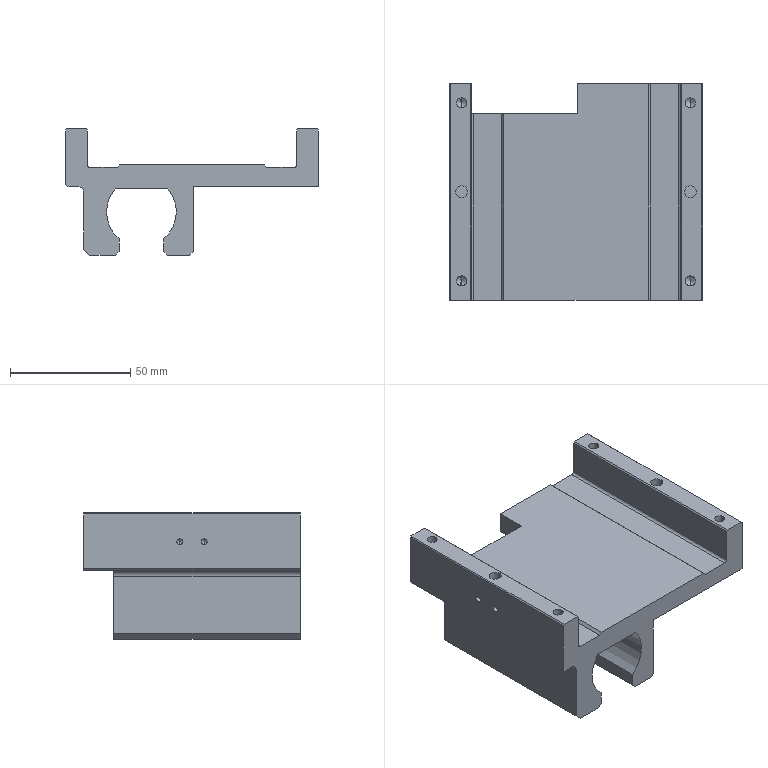Part | SolidWorks | features BaseBody 1 | 1 solid | 81 faces | box 105 x 90 x 52.5 mm | volume 149012 mm3 | plane 36 | cylinder 27 | cone 18 | commonest cylinder face diameters 2.5 x8 4.2 x8 5 x5 2 x2 3.3 x2 29 x2